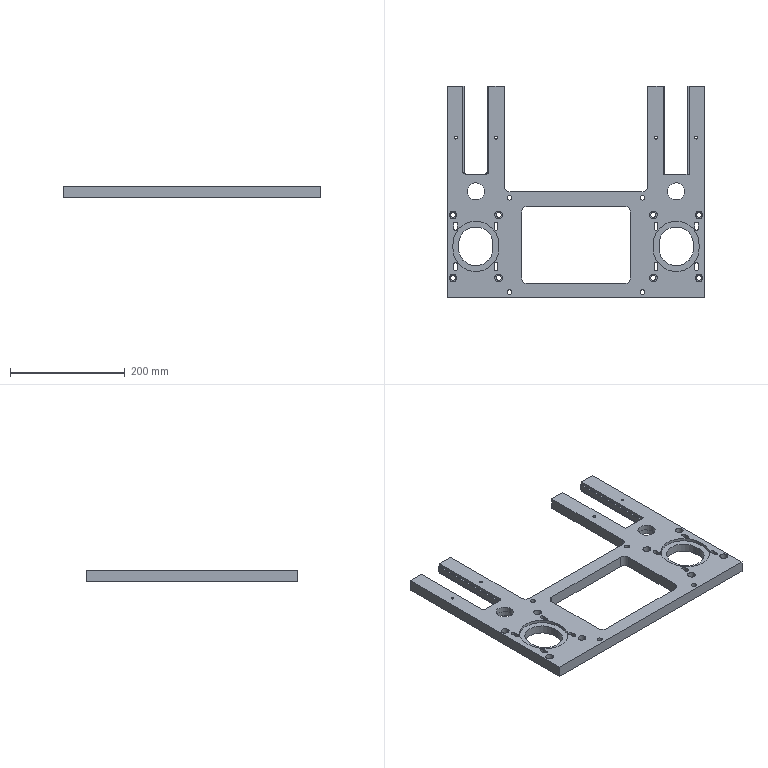Part | STEP file | A14-010 | 1 solid | 166 faces | box 450 x 370 x 20 mm | volume 1407992 mm3 | cylinder 92 | plane 74 | commonest cylinder face diameters 8.5 x24 6.5 x16 13.5 x16 5 x8 10 x6 20 x6